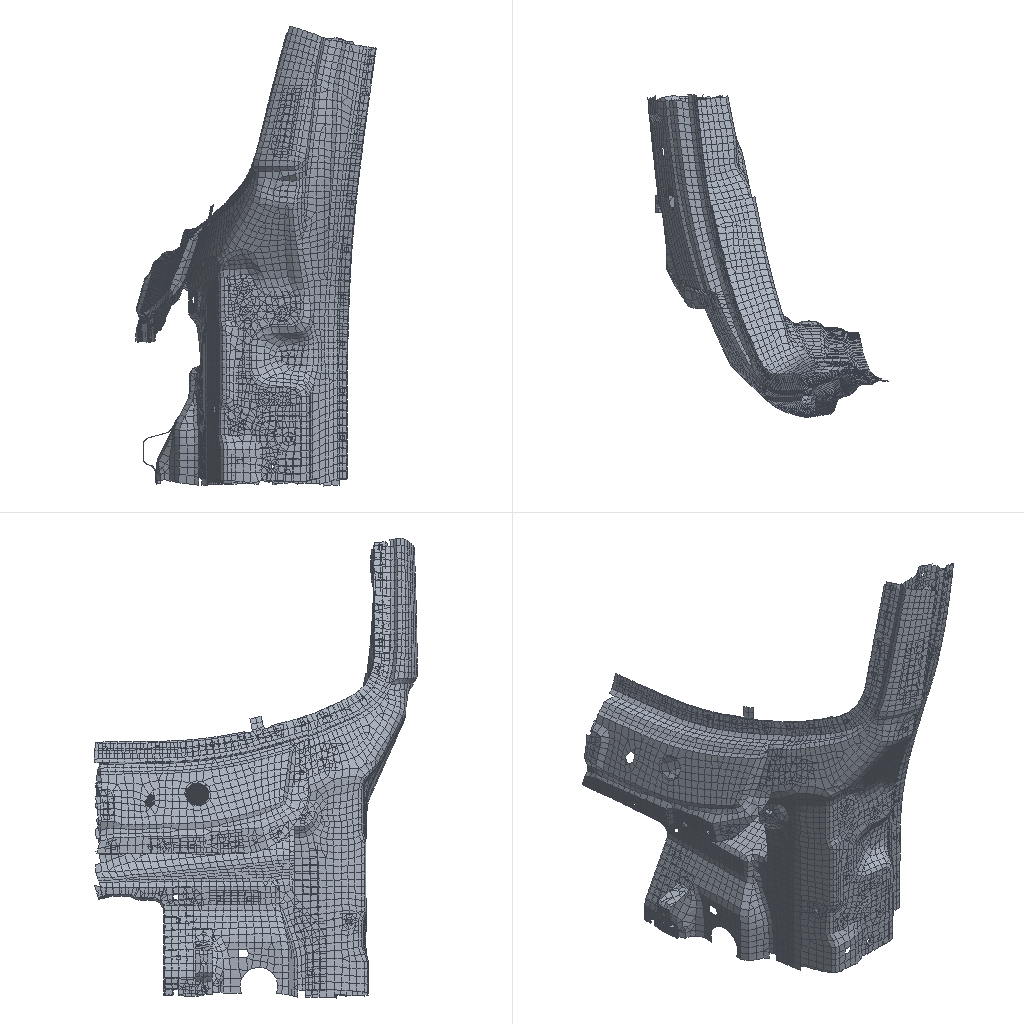Simulation study | nastran
Set-up summary:
category,name,step,type,value,unit,region
solver,nx_nastran
units,not stated in the deck,,not stated
analysis,deck,,static,static
analysis,solution,,SOL,101
load_step,SUBCASE 2,2,SUBCASE,SPC=2 LOAD=5
load_step,SUBCASE 3,3,SUBCASE,SPC=2 LOAD=3
load_step,SUBCASE 4,4,SUBCASE,SPC=2 LOAD=4
load_step,requested,,,3
mesh,nodes,,,10845
mesh,elements,,,9853
element_type,CHEXA,,solid,86
element_type,CQUAD4,,shell,8980
element_type,CTRIA3,,shell,787
load,load commands in deck,,count,3
bc,support commands in deck,,count,364
check,setup vs results,,match,"every grid point's frame and coordinates and every element id; grid points of CHEXA, CQUAD4, CTRIA3 elements"
Nastran input file, long lists of numbers shortened:
$$------------------------------------------------------------------------------$
$$                                                                              $
$$ NASTRAN Input Deck Generated by HyperMesh Version  :10.0buil                 $
$$ Generated using HyperMesh-Nastran Template Version : 10.0build60
$$                                                                              $
$$   Template:  general                                                         $
$$                                                                              $
$$------------------------------------------------------------------------------$
$$------------------------------------------------------------------------------$
$$                      Executive Control Cards                                 $
$$------------------------------------------------------------------------------$
SOL 101
CEND
$$------------------------------------------------------------------------------$
$$                      Case Control Cards                                      $
$$------------------------------------------------------------------------------$
  DISPLACEMENT = ALL
  ESE = ALL
$
$HMNAME LOADSTEP               2"fz"
SUBCASE       2
  LABEL=   fz
  SPC =        2
  LOAD =        5
$
$HMNAME LOADSTEP               3"fx"
SUBCASE       3
  LABEL=   fx
  SPC =        2
  LOAD =        3
$
$HMNAME LOADSTEP               4"fy"
SUBCASE       4
  LABEL=   fy
  SPC =        2
  LOAD =        4
$$------------------------------------------------------------------------------$
$$                      Bulk Data Cards                                         $
$$------------------------------------------------------------------------------$
BEGIN BULK
PARAM,POST,-1
$$
$$  GRID Data
$$
GRID         150        -903.017-1033.041012.706
GRID         536        -985.883-1013.11735.4542
$ (10843 more lines like these left out)
$$
$$  SPOINT Data
$$
$$
$$------------------------------------------------------------------------------$
$$             Group Definitions                                                $
$$------------------------------------------------------------------------------$
$$
$$ RBE2 Elements - Multiple dependent nodes
$$
RBE2     101461184100703  123456    1053  618882  618883  618901  618903+
+         618904  618942  618943  618962  618963  618974  618975  621939+
+         621940  621947  621948  623188  623195  631238  631239  641137+
+         641151  642040  642041  642042  642043  642044  642045  642046+
+         642047  648139  648140  648160  648200  648201  648208  648209+
+         648231  648232  648240  648241  648317  648318  649091  649092+
+         649099  649100  649296  649298  649299  649300  649301  649303+
+        3748720 3748721 3748931 3748932 3750121 3750122 3750126 3750127+
+        3750192 3750239 3750610 3750611 3750622 3750623 3750651 3750652+
+        3750657 3754737 3754738 3754748 3754749840989048409890584099220+
+       8409922884099232840992338409954384099544840995778409957884099582+
+       8409958384099622840996238409976484099765840997918409979284100526+
+       84100527
$
$HMMOVE 84022690
$        1014611
$
$
$  RBE3 Elements
$
RBE3      327795         3756945  1234560.741826     123  6410970.130387+
+            123  6233140.019103     123  6233130.108684     123  623320
RBE3      327796         3756946  1234560.103694     123  6410970.024184+
+            123  6233140.164933     123  6233130.70719      123  623320
$ (1364 more lines like these left out)
$
$HMMOVE 57005012
$         327795THRU      327798  327800THRU      327807  327809THRU      327816
$         327818THRU      327825  327827THRU      327834  327836THRU      327843
$ (39 more lines like these left out)
CTRIA3    170855      12   87448   87447   87413
CTRIA3    170898      12   87483   87526   87523
$ (785 more lines like these left out)
$
$HMMOVE       20
$         170855  170898  170901  170912  170962  170964  170969  170973  171049
$         171064THRU      171066  171072  171088  171093THRU      171094  171096
$ (124 more lines like these left out)
CQUAD4    192149      12   88275   88714   88754   88276
CQUAD4    192150      12   88276   88754   88753   88277
$ (8978 more lines like these left out)
$
$HMMOVE       20
$         192149THRU      192152  178431  178465THRU      178470  178479THRU
$         178480  178482  178490  178534THRU      178537  178539THRU      178543
$ (327 more lines like these left out)
CHEXA     327799      10 3756945 3756946 3756947 3756948 3756949 3756950+
+        3756951 3756952
CHEXA     327808      10 3756954 3756955 3756956 3756957 3756958 3756959+
+        3756960 3756961
$ (168 more lines like these left out)
$
$HMMOVE 57005011
$         327799  327808  327817  327826  327835  327844  327853  327862  327871
$         327880  327961  327970  327979  327988  327997  328006  328015  328024
$ (79 more lines like these left out)
PSHELL         9       20.8            2               2
$
$HMNAME PROP                  10"120" 4
$HWCOLOR PROP                 10       3
PSHELL        10       21.2            2               2
$
$HMNAME PROP                  12"100" 4
$HWCOLOR PROP                 12       3
PSHELL        12       21.0            2               2
$
$HMNAME PROP                   5"150" 4
$HWCOLOR PROP                  5       3
PSHELL         5       21.5            2               2
$$
$$  PSOLID Data
$
$HMNAME PROP                  10"spot.1" 5
$HWCOLOR PROP                 10       3
PSOLID        10       2
$$
$$------------------------------------------------------------------------------$
$$                      Material Definition Cards                               $
$$------------------------------------------------------------------------------$
$$--------------------------------------------------------------
$$ HYPERMESH TAGS
$$--------------------------------------------------------------
$$BEGIN TAGS
$$END TAGS
$$
$$  MAT1 Data
$
$HMNAME MAT                    2"steel.1" "MAT1"
$HWCOLOR MAT                   2       3
MAT1           2210000.0        0.3     7.80E-09
$$
$$
$$
$$------------------------------------------------------------------------------$
$ (42 more lines like these left out)
SPC            2  647276  1234560.0
SPC            2  647275  1234560.0
SPC            2  647270  1234560.0
SPC            2  647269  1234560.0
$ (360 more lines like these left out)
$$
$$  FORCE Data
$$
FORCE          384100703       01.0     140.0   0.0     0.0
FORCE          484100703       01.0     0.0     320.0   0.0
FORCE          584100703       01.0     0.0     0.0     140.0
$HMASSEM      28       4 5300010
$HMASSEM_IDS          20      21      22      24      25      26
$HMASSEM 5400100       7 sidebody_L
$HMASSEM_IDS    840226895400303054003020540011105400112054003010
$
ENDDATA
Results summary:
result,analysis,,,static
result,last_loadstep,,,3
result,primary field,,,displacements
result,max displacement,,,0.5322,model units